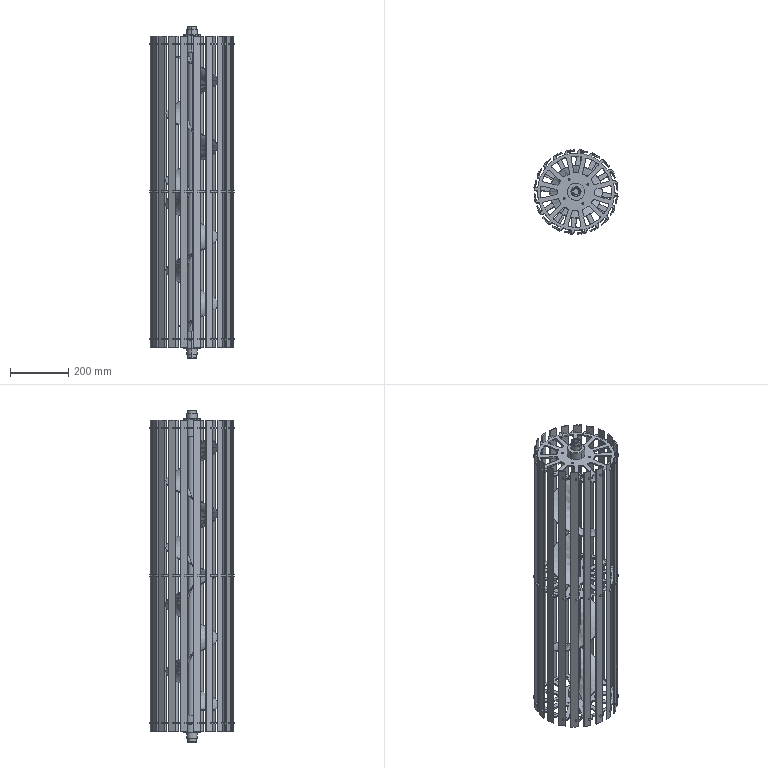Part | SolidWorks | features ReferencePattern 19, CompositeCurve 2, LocalCirPattern 1 | 28 solids | 928 faces | box 289.417 x 289.417 x 1144 mm | volume 3340527 mm3 | plane 459 | cylinder 442 | cone 19 | spline 8 | commonest cylinder face diameters 10 x180 22 x75 265 x60 245 x39 130 x26 6.5 x16